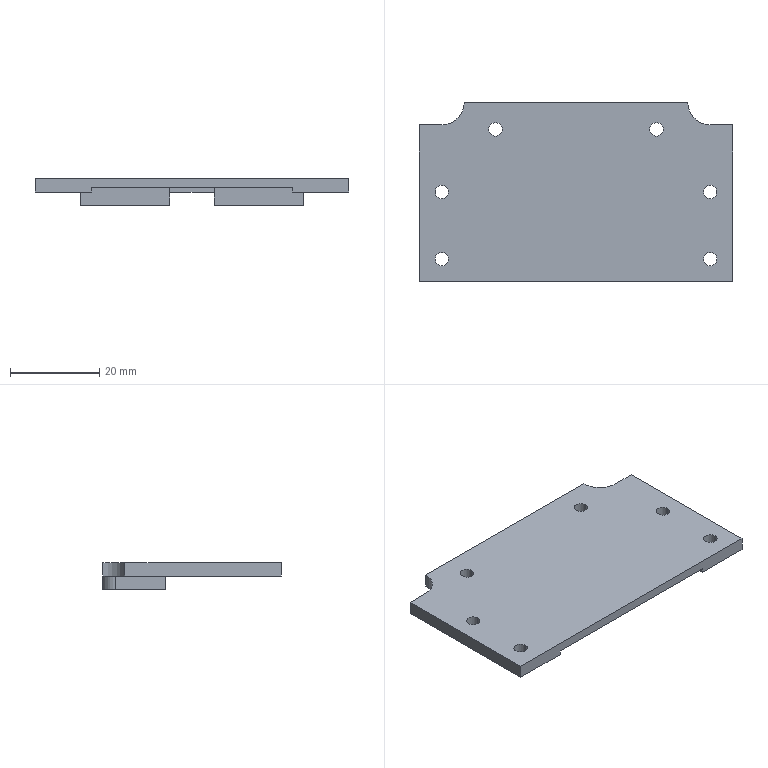Part | SolidWorks | features ICE 2, MBimport 1 | 1 solid | 48 faces | box 70 x 40 x 6 mm | volume 8316 mm3 | plane 28 | cylinder 20 | commonest cylinder face diameters 3 x16 6 x2 10 x2
STEP:
#1=CARTESIAN_POINT('',(-8.5,14.,1.));
#2=VERTEX_POINT('',#1);
#3=CARTESIAN_POINT('',(-11.5,14.,1.));
#4=VERTEX_POINT('',#3);
#5=CARTESIAN_POINT('',(-10.,14.,1.));
#6=DIRECTION('',(0.,0.,-1.));
#7=DIRECTION('',(-1.,0.,0.));
#8=AXIS2_PLACEMENT_3D('',#5,#6,#7);
#9=CIRCLE('',#8,1.5);
#10=EDGE_CURVE('',#2,#4,#9,.T.);
#11=ORIENTED_EDGE('',*,*,#10,.F.);
#12=CARTESIAN_POINT('',(-8.5,14.,-3.));
#13=VERTEX_POINT('',#12);
#14=CARTESIAN_POINT('',(-8.5,14.,3.002));
#15=DIRECTION('',(0.,0.,-1.));
#16=VECTOR('',#15,1000.);
#17=LINE('',#14,#16);
#18=EDGE_CURVE('',#2,#13,#17,.T.);
#19=ORIENTED_EDGE('',*,*,#18,.T.);
#20=CARTESIAN_POINT('',(-11.5,14.,-3.));
#21=VERTEX_POINT('',#20);
#22=CARTESIAN_POINT('',(-10.,14.,-3.));
#23=DIRECTION('',(0.,0.,1.));
#24=DIRECTION('',(-1.,0.,0.));
#25=AXIS2_PLACEMENT_3D('',#22,#23,#24);
#26=CIRCLE('',#25,1.5);
#27=EDGE_CURVE('',#21,#13,#26,.T.);
#28=ORIENTED_EDGE('',*,*,#27,.F.);
#29=CARTESIAN_POINT('',(-11.5,14.,3.002));
#30=DIRECTION('',(0.,0.,-1.));
#31=VECTOR('',#30,1000.);
#32=LINE('',#29,#31);
#33=EDGE_CURVE('',#4,#21,#32,.T.);
#34=ORIENTED_EDGE('',*,*,#33,.F.);
#35=EDGE_LOOP('',(#11,#19,#28,#34));
#36=FACE_OUTER_BOUND('',#35,.T.);
#37=CARTESIAN_POINT('',(-10.,14.,3.002));
#38=DIRECTION('',(0.,0.,-1.));
#39=DIRECTION('',(-1.,0.,0.));
#40=AXIS2_PLACEMENT_3D('',#37,#38,#39);
#41=CYLINDRICAL_SURFACE('',#40,1.5);
#42=ADVANCED_FACE('',(#36),#41,.F.);
#43=CARTESIAN_POINT('',(8.5,14.,1.));
#44=VERTEX_POINT('',#43);
#45=CARTESIAN_POINT('',(11.5,14.,1.));
#46=VERTEX_POINT('',#45);
#47=CARTESIAN_POINT('',(10.,14.,1.));
#48=DIRECTION('',(0.,0.,1.));
#49=DIRECTION('',(-1.,0.,0.));
#50=AXIS2_PLACEMENT_3D('',#47,#48,#49);
#51=CIRCLE('',#50,1.5);
#52=EDGE_CURVE('',#44,#46,#51,.T.);
#53=ORIENTED_EDGE('',*,*,#52,.T.);
#54=CARTESIAN_POINT('',(11.5,14.,-3.));
#55=VERTEX_POINT('',#54);
#56=CARTESIAN_POINT('',(11.5,14.,3.002));
#57=DIRECTION('',(0.,0.,-1.));
#58=VECTOR('',#57,1000.);
#59=LINE('',#56,#58);
#60=EDGE_CURVE('',#46,#55,#59,.T.);
#61=ORIENTED_EDGE('',*,*,#60,.T.);
#62=CARTESIAN_POINT('',(8.5,14.,-3.));
#63=VERTEX_POINT('',#62);
#64=CARTESIAN_POINT('',(10.,14.,-3.));
#65=DIRECTION('',(0.,0.,-1.));
#66=DIRECTION('',(-1.,0.,0.));
#67=AXIS2_PLACEMENT_3D('',#64,#65,#66);
#68=CIRCLE('',#67,1.5);
#69=EDGE_CURVE('',#55,#63,#68,.T.);
#70=ORIENTED_EDGE('',*,*,#69,.T.);
#71=CARTESIAN_POINT('',(8.5,14.,3.002));
#72=DIRECTION('',(0.,0.,-1.));
#73=VECTOR('',#72,1000.);
#74=LINE('',#71,#73);
#75=EDGE_CURVE('',#44,#63,#74,.T.);
#76=ORIENTED_EDGE('',*,*,#75,.F.);
#77=EDGE_LOOP('',(#53,#61,#70,#76));
#78=FACE_OUTER_BOUND('',#77,.T.);
#79=CARTESIAN_POINT('',(10.,14.,3.002));
#80=DIRECTION('',(0.,0.,-1.));
#81=DIRECTION('',(-1.,0.,0.));
#82=AXIS2_PLACEMENT_3D('',#79,#80,#81);
#83=CYLINDRICAL_SURFACE('',#82,1.5);
#84=ADVANCED_FACE('',(#78),#83,.F.);
#85=CARTESIAN_POINT('',(-22.5,6.,1.));
#86=VERTEX_POINT('',#85);
#87=CARTESIAN_POINT('',(-5.,6.,1.));
#88=VERTEX_POINT('',#87);
#89=CARTESIAN_POINT('',(-22.5,6.,1.));
#90=DIRECTION('',(1.,0.,0.));
#91=VECTOR('',#90,1000.);
#92=LINE('',#89,#91);
#93=EDGE_CURVE('',#86,#88,#92,.T.);
#94=ORIENTED_EDGE('',*,*,#93,.T.);
#95=CARTESIAN_POINT('',(-5.,15.,1.));
#96=VERTEX_POINT('',#95);
#97=CARTESIAN_POINT('',(-5.,0.,1.));
#98=DIRECTION('',(0.,-1.,0.));
#99=VECTOR('',#98,1000.);
#100=LINE('',#97,#99);
#101=EDGE_CURVE('',#96,#88,#100,.T.);
#102=ORIENTED_EDGE('',*,*,#101,.F.);
#103=CARTESIAN_POINT('',(5.,15.,1.));
#104=VERTEX_POINT('',#103);
#105=CARTESIAN_POINT('',(-15.,15.,1.));
#106=DIRECTION('',(1.,0.,0.));
#107=VECTOR('',#106,1000.);
#108=LINE('',#105,#107);
#109=EDGE_CURVE('',#96,#104,#108,.T.);
#110=ORIENTED_EDGE('',*,*,#109,.T.);
#111=CARTESIAN_POINT('',(5.,6.,1.));
#112=VERTEX_POINT('',#111);
#113=CARTESIAN_POINT('',(5.,0.,1.));
#114=DIRECTION('',(0.,-1.,0.));
#115=VECTOR('',#114,1000.);
#116=LINE('',#113,#115);
#117=EDGE_CURVE('',#104,#112,#116,.T.);
#118=ORIENTED_EDGE('',*,*,#117,.T.);
#119=CARTESIAN_POINT('',(22.5,6.,1.));
#120=VERTEX_POINT('',#119);
#121=CARTESIAN_POINT('',(22.5,6.,1.));
#122=DIRECTION('',(-1.,0.,0.));
#123=VECTOR('',#122,1000.);
#124=LINE('',#121,#123);
#125=EDGE_CURVE('',#120,#112,#124,.T.);
#126=ORIENTED_EDGE('',*,*,#125,.F.);
#127=CARTESIAN_POINT('',(22.5,-20.,1.));
#128=VERTEX_POINT('',#127);
#129=CARTESIAN_POINT('',(22.5,6.,1.));
#130=DIRECTION('',(0.,-1.,0.));
#131=VECTOR('',#130,1000.);
#132=LINE('',#129,#131);
#133=EDGE_CURVE('',#120,#128,#132,.T.);
#134=ORIENTED_EDGE('',*,*,#133,.T.);
#135=CARTESIAN_POINT('',(-22.5,-20.,1.));
#136=VERTEX_POINT('',#135);
#137=CARTESIAN_POINT('',(22.5,-20.,1.));
#138=DIRECTION('',(-1.,0.,0.));
#139=VECTOR('',#138,1000.);
#140=LINE('',#137,#139);
#141=EDGE_CURVE('',#128,#136,#140,.T.);
#142=ORIENTED_EDGE('',*,*,#141,.T.);
#143=CARTESIAN_POINT('',(-22.5,-20.,1.));
#144=DIRECTION('',(0.,1.,0.));
#145=VECTOR('',#144,1000.);
#146=LINE('',#143,#145);
#147=EDGE_CURVE('',#136,#86,#146,.T.);
#148=ORIENTED_EDGE('',*,*,#147,.T.);
#149=EDGE_LOOP('',(#94,#102,#110,#118,#126,#134,#142,#148));
#150=FACE_OUTER_BOUND('',#149,.T.);
#151=CARTESIAN_POINT('',(0.,0.,1.));
#152=DIRECTION('',(0.,0.,-1.));
#153=DIRECTION('',(-1.,0.,0.));
#154=AXIS2_PLACEMENT_3D('',#151,#152,#153);
#155=PLANE('',#154);
#156=ADVANCED_FACE('',(#150),#155,.T.);
#157=CARTESIAN_POINT('',(-5.,15.,0.));
#158=VERTEX_POINT('',#157);
#159=CARTESIAN_POINT('',(-5.,20.,0.));
#160=VERTEX_POINT('',#159);
#161=CARTESIAN_POINT('',(-5.,0.,0.));
#162=DIRECTION('',(0.,1.,0.));
#163=VECTOR('',#162,1000.);
#164=LINE('',#161,#163);
#165=EDGE_CURVE('',#158,#160,#164,.T.);
#166=ORIENTED_EDGE('',*,*,#165,.T.);
#167=CARTESIAN_POINT('',(5.,20.,0.));
#168=VERTEX_POINT('',#167);
#169=CARTESIAN_POINT('',(15.,20.,0.));
#170=DIRECTION('',(-1.,0.,0.));
#171=VECTOR('',#170,1000.);
#172=LINE('',#169,#171);
#173=EDGE_CURVE('',#168,#160,#172,.T.);
#174=ORIENTED_EDGE('',*,*,#173,.F.);
#175=CARTESIAN_POINT('',(5.,15.,0.));
#176=VERTEX_POINT('',#175);
#177=CARTESIAN_POINT('',(5.,0.,0.));
#178=DIRECTION('',(0.,1.,0.));
#179=VECTOR('',#178,1000.);
#180=LINE('',#177,#179);
#181=EDGE_CURVE('',#176,#168,#180,.T.);
#182=ORIENTED_EDGE('',*,*,#181,.F.);
#183=CARTESIAN_POINT('',(-15.,15.,0.));
#184=DIRECTION('',(1.,0.,0.));
#185=VECTOR('',#184,1000.);
#186=LINE('',#183,#185);
#187=EDGE_CURVE('',#158,#176,#186,.T.);
#188=ORIENTED_EDGE('',*,*,#187,.F.);
#189=EDGE_LOOP('',(#166,#174,#182,#188));
#190=FACE_OUTER_BOUND('',#189,.T.);
#191=CARTESIAN_POINT('',(0.,0.,0.));
#192=DIRECTION('',(0.,0.,1.));
#193=DIRECTION('',(0.,-1.,0.));
#194=AXIS2_PLACEMENT_3D('',#191,#192,#193);
#195=PLANE('',#194);
#196=ADVANCED_FACE('',(#190),#195,.F.);
#197=CARTESIAN_POINT('',(-5.,15.,3.002));
#198=DIRECTION('',(0.,0.,-1.));
#199=VECTOR('',#198,1000.);
#200=LINE('',#197,#199);
#201=EDGE_CURVE('',#96,#158,#200,.T.);
#202=ORIENTED_EDGE('',*,*,#201,.T.);
#203=ORIENTED_EDGE('',*,*,#187,.T.);
#204=CARTESIAN_POINT('',(5.,15.,3.002));
#205=DIRECTION('',(0.,0.,-1.));
#206=VECTOR('',#205,1000.);
#207=LINE('',#204,#206);
#208=EDGE_CURVE('',#104,#176,#207,.T.);
#209=ORIENTED_EDGE('',*,*,#208,.F.);
#210=ORIENTED_EDGE('',*,*,#109,.F.);
#211=EDGE_LOOP('',(#202,#203,#209,#210));
#212=FACE_OUTER_BOUND('',#211,.T.);
#213=CARTESIAN_POINT('',(-22.5,15.,0.));
#214=DIRECTION('',(0.,1.,0.));
#215=DIRECTION('',(1.,0.,0.));
#216=AXIS2_PLACEMENT_3D('',#213,#214,#215);
#217=PLANE('',#216);
#218=ADVANCED_FACE('',(#212),#217,.F.);
#219=CARTESIAN_POINT('',(-31.5,0.,0.));
#220=VERTEX_POINT('',#219);
#221=CARTESIAN_POINT('',(-28.5,0.,0.));
#222=VERTEX_POINT('',#221);
#223=CARTESIAN_POINT('',(-30.,0.,0.));
#224=DIRECTION('',(0.,0.,1.));
#225=DIRECTION('',(-1.,0.,0.));
#226=AXIS2_PLACEMENT_3D('',#223,#224,#225);
#227=CIRCLE('',#226,1.5);
#228=EDGE_CURVE('',#220,#222,#227,.T.);
#229=ORIENTED_EDGE('',*,*,#228,.T.);
#230=CARTESIAN_POINT('',(-30.,0.,0.));
#231=DIRECTION('',(0.,0.,1.));
#232=DIRECTION('',(1.,0.,0.));
#233=AXIS2_PLACEMENT_3D('',#230,#231,#232);
#234=CIRCLE('',#233,1.5);
#235=EDGE_CURVE('',#222,#220,#234,.T.);
#236=ORIENTED_EDGE('',*,*,#235,.T.);
#237=EDGE_LOOP('',(#229,#236));
#238=FACE_BOUND('',#237,.T.);
#239=CARTESIAN_POINT('',(-25.,6.,0.));
#240=VERTEX_POINT('',#239);
#241=CARTESIAN_POINT('',(-22.5,6.,0.));
#242=VERTEX_POINT('',#241);
#243=CARTESIAN_POINT('',(-25.,6.,0.));
#244=DIRECTION('',(1.,0.,0.));
#245=VECTOR('',#244,1000.);
#246=LINE('',#243,#245);
#247=EDGE_CURVE('',#240,#242,#246,.T.);
#248=ORIENTED_EDGE('',*,*,#247,.T.);
#249=CARTESIAN_POINT('',(-22.5,-20.,0.));
#250=VERTEX_POINT('',#249);
#251=CARTESIAN_POINT('',(-22.5,-17.,0.));
#252=DIRECTION('',(0.,1.,0.));
#253=VECTOR('',#252,1000.);
#254=LINE('',#251,#253);
#255=EDGE_CURVE('',#250,#242,#254,.T.);
#256=ORIENTED_EDGE('',*,*,#255,.F.);
#257=CARTESIAN_POINT('',(-35.,-20.,0.));
#258=VERTEX_POINT('',#257);
#259=CARTESIAN_POINT('',(-35.,-20.,0.));
#260=DIRECTION('',(-1.,0.,0.));
#261=VECTOR('',#260,1000.);
#262=LINE('',#259,#261);
#263=EDGE_CURVE('',#250,#258,#262,.T.);
#264=ORIENTED_EDGE('',*,*,#263,.T.);
#265=CARTESIAN_POINT('',(-35.,15.,0.));
#266=VERTEX_POINT('',#265);
#267=CARTESIAN_POINT('',(-35.,15.,0.));
#268=DIRECTION('',(0.,-1.,0.));
#269=VECTOR('',#268,1000.);
#270=LINE('',#267,#269);
#271=EDGE_CURVE('',#266,#258,#270,.T.);
#272=ORIENTED_EDGE('',*,*,#271,.F.);
#273=CARTESIAN_POINT('',(-30.,15.,0.));
#274=VERTEX_POINT('',#273);
#275=CARTESIAN_POINT('',(-35.,15.,0.));
#276=DIRECTION('',(1.,0.,0.));
#277=VECTOR('',#276,1000.);
#278=LINE('',#275,#277);
#279=EDGE_CURVE('',#266,#274,#278,.T.);
#280=ORIENTED_EDGE('',*,*,#279,.T.);
#281=CARTESIAN_POINT('',(-25.,20.,0.));
#282=VERTEX_POINT('',#281);
#283=CARTESIAN_POINT('',(-30.,20.,0.));
#284=DIRECTION('',(0.,0.,1.));
#285=DIRECTION('',(0.,-1.,0.));
#286=AXIS2_PLACEMENT_3D('',#283,#284,#285);
#287=CIRCLE('',#286,5.);
#288=EDGE_CURVE('',#274,#282,#287,.T.);
#289=ORIENTED_EDGE('',*,*,#288,.T.);
#290=CARTESIAN_POINT('',(-22.,20.,0.));
#291=VERTEX_POINT('',#290);
#292=CARTESIAN_POINT('',(-22.,20.,0.));
#293=DIRECTION('',(-1.,0.,0.));
#294=VECTOR('',#293,1000.);
#295=LINE('',#292,#294);
#296=EDGE_CURVE('',#291,#282,#295,.T.);
#297=ORIENTED_EDGE('',*,*,#296,.F.);
#298=CARTESIAN_POINT('',(-25.,17.,0.));
#299=VERTEX_POINT('',#298);
#300=CARTESIAN_POINT('',(-22.,17.,0.));
#301=DIRECTION('',(0.,0.,1.));
#302=DIRECTION('',(0.,1.,0.));
#303=AXIS2_PLACEMENT_3D('',#300,#301,#302);
#304=CIRCLE('',#303,3.);
#305=EDGE_CURVE('',#291,#299,#304,.T.);
#306=ORIENTED_EDGE('',*,*,#305,.T.);
#307=CARTESIAN_POINT('',(-25.,17.,0.));
#308=DIRECTION('',(0.,-1.,0.));
#309=VECTOR('',#308,1000.);
#310=LINE('',#307,#309);
#311=EDGE_CURVE('',#299,#240,#310,.T.);
#312=ORIENTED_EDGE('',*,*,#311,.T.);
#313=EDGE_LOOP('',(#248,#256,#264,#272,#280,#289,#297,#306,#312));
#314=FACE_OUTER_BOUND('',#313,.T.);
#315=CARTESIAN_POINT('',(-31.5,-15.,0.));
#316=VERTEX_POINT('',#315);
#317=CARTESIAN_POINT('',(-28.5,-15.,0.));
#318=VERTEX_POINT('',#317);
#319=CARTESIAN_POINT('',(-30.,-15.,0.));
#320=DIRECTION('',(0.,0.,-1.));
#321=DIRECTION('',(1.,0.,0.));
#322=AXIS2_PLACEMENT_3D('',#319,#320,#321);
#323=CIRCLE('',#322,1.5);
#324=EDGE_CURVE('',#316,#318,#323,.T.);
#325=ORIENTED_EDGE('',*,*,#324,.F.);
#326=CARTESIAN_POINT('',(-30.,-15.,0.));
#327=DIRECTION('',(0.,0.,-1.));
#328=DIRECTION('',(1.,0.,0.));
#329=AXIS2_PLACEMENT_3D('',#326,#327,#328);
#330=CIRCLE('',#329,1.5);
#331=EDGE_CURVE('',#318,#316,#330,.T.);
#332=ORIENTED_EDGE('',*,*,#331,.F.);
#333=EDGE_LOOP('',(#325,#332));
#334=FACE_BOUND('',#333,.T.);
#335=CARTESIAN_POINT('',(0.,0.,0.));
#336=DIRECTION('',(0.,0.,1.));
#337=DIRECTION('',(0.,-1.,0.));
#338=AXIS2_PLACEMENT_3D('',#335,#336,#337);
#339=PLANE('',#338);
#340=ADVANCED_FACE('',(#238,#314,#334),#339,.F.);
#341=ORIENTED_EDGE('',*,*,#228,.F.);
#342=CARTESIAN_POINT('',(-31.5,0.,3.));
#343=VERTEX_POINT('',#342);
#344=CARTESIAN_POINT('',(-31.5,0.,0.));
#345=DIRECTION('',(0.,0.,1.));
#346=VECTOR('',#345,1000.);
#347=LINE('',#344,#346);
#348=EDGE_CURVE('',#220,#343,#347,.T.);
#349=ORIENTED_EDGE('',*,*,#348,.T.);
#350=CARTESIAN_POINT('',(-28.5,0.,3.));
#351=VERTEX_POINT('',#350);
#352=CARTESIAN_POINT('',(-30.,0.,3.));
#353=DIRECTION('',(0.,0.,1.));
#354=DIRECTION('',(-1.,0.,0.));
#355=AXIS2_PLACEMENT_3D('',#352,#353,#354);
#356=CIRCLE('',#355,1.5);
#357=EDGE_CURVE('',#343,#351,#356,.T.);
#358=ORIENTED_EDGE('',*,*,#357,.T.);
#359=CARTESIAN_POINT('',(-28.5,0.,0.));
#360=DIRECTION('',(0.,0.,1.));
#361=VECTOR('',#360,1000.);
#362=LINE('',#359,#361);
#363=EDGE_CURVE('',#222,#351,#362,.T.);
#364=ORIENTED_EDGE('',*,*,#363,.F.);
#365=EDGE_LOOP('',(#341,#349,#358,#364));
#366=FACE_OUTER_BOUND('',#365,.T.);
#367=CARTESIAN_POINT('',(-30.,0.,0.));
#368=DIRECTION('',(0.,0.,-1.));
#369=DIRECTION('',(1.,0.,0.));
#370=AXIS2_PLACEMENT_3D('',#367,#368,#369);
#371=CYLINDRICAL_SURFACE('',#370,1.5);
#372=ADVANCED_FACE('',(#366),#371,.F.);
#373=CARTESIAN_POINT('',(-30.,0.,3.));
#374=DIRECTION('',(0.,0.,1.));
#375=DIRECTION('',(1.,0.,0.));
#376=AXIS2_PLACEMENT_3D('',#373,#374,#375);
#377=CIRCLE('',#376,1.5);
#378=EDGE_CURVE('',#351,#343,#377,.T.);
#379=ORIENTED_EDGE('',*,*,#378,.T.);
#380=ORIENTED_EDGE('',*,*,#348,.F.);
#381=ORIENTED_EDGE('',*,*,#235,.F.);
#382=ORIENTED_EDGE('',*,*,#363,.T.);
#383=EDGE_LOOP('',(#379,#380,#381,#382));
#384=FACE_OUTER_BOUND('',#383,.T.);
#385=CARTESIAN_POINT('',(-30.,0.,0.));
#386=DIRECTION('',(0.,0.,-1.));
#387=DIRECTION('',(1.,0.,0.));
#388=AXIS2_PLACEMENT_3D('',#385,#386,#387);
#389=CYLINDRICAL_SURFACE('',#388,1.5);
#390=ADVANCED_FACE('',(#384),#389,.F.);
#391=CARTESIAN_POINT('',(-25.,6.,-3.));
#392=VERTEX_POINT('',#391);
#393=CARTESIAN_POINT('',(-5.,6.,-3.));
#394=VERTEX_POINT('',#393);
#395=CARTESIAN_POINT('',(-25.,6.,-3.));
#396=DIRECTION('',(1.,0.,0.));
#397=VECTOR('',#396,1000.);
#398=LINE('',#395,#397);
#399=EDGE_CURVE('',#392,#394,#398,.T.);
#400=ORIENTED_EDGE('',*,*,#399,.T.);
#401=CARTESIAN_POINT('',(-5.,6.,3.002));
#402=DIRECTION('',(0.,0.,-1.));
#403=VECTOR('',#402,1000.);
#404=LINE('',#401,#403);
#405=EDGE_CURVE('',#88,#394,#404,.T.);
#406=ORIENTED_EDGE('',*,*,#405,.F.);
#407=ORIENTED_EDGE('',*,*,#93,.F.);
#408=CARTESIAN_POINT('',(-22.5,6.,1.));
#409=DIRECTION('',(0.,0.,-1.));
#410=VECTOR('',#409,1000.);
#411=LINE('',#408,#410);
#412=EDGE_CURVE('',#86,#242,#411,.T.);
#413=ORIENTED_EDGE('',*,*,#412,.T.);
#414=ORIENTED_EDGE('',*,*,#247,.F.);
#415=CARTESIAN_POINT('',(-25.,6.,0.));
#416=DIRECTION('',(0.,0.,-1.));
#417=VECTOR('',#416,1000.);
#418=LINE('',#415,#417);
#419=EDGE_CURVE('',#240,#392,#418,.T.);
#420=ORIENTED_EDGE('',*,*,#419,.T.);
#421=EDGE_LOOP('',(#400,#406,#407,#413,#414,#420));
#422=FACE_OUTER_BOUND('',#421,.T.);
#423=CARTESIAN_POINT('',(-25.,6.,1.));
#424=DIRECTION('',(0.,1.,0.));
#425=DIRECTION('',(1.,0.,0.));
#426=AXIS2_PLACEMENT_3D('',#423,#424,#425);
#427=PLANE('',#426);
#428=ADVANCED_FACE('',(#422),#427,.F.);
#429=CARTESIAN_POINT('',(-22.5,-20.,-6.));
#430=DIRECTION('',(0.,0.,1.));
#431=VECTOR('',#430,1000.);
#432=LINE('',#429,#431);
#433=EDGE_CURVE('',#250,#136,#432,.T.);
#434=ORIENTED_EDGE('',*,*,#433,.F.);
#435=ORIENTED_EDGE('',*,*,#255,.T.);
#436=ORIENTED_EDGE('',*,*,#412,.F.);
#437=ORIENTED_EDGE('',*,*,#147,.F.);
#438=EDGE_LOOP('',(#434,#435,#436,#437));
#439=FACE_OUTER_BOUND('',#438,.T.);
#440=CARTESIAN_POINT('',(-22.5,-20.,0.));
#441=DIRECTION('',(-1.,0.,0.));
#442=DIRECTION('',(0.,1.,0.));
#443=AXIS2_PLACEMENT_3D('',#440,#441,#442);
#444=PLANE('',#443);
#445=ADVANCED_FACE('',(#439),#444,.F.);
#446=ORIENTED_EDGE('',*,*,#271,.T.);
#447=CARTESIAN_POINT('',(-35.,-20.,3.));
#448=VERTEX_POINT('',#447);
#449=CARTESIAN_POINT('',(-35.,-20.,3.));
#450=DIRECTION('',(0.,0.,-1.));
#451=VECTOR('',#450,1000.);
#452=LINE('',#449,#451);
#453=EDGE_CURVE('',#448,#258,#452,.T.);
#454=ORIENTED_EDGE('',*,*,#453,.F.);
#455=CARTESIAN_POINT('',(-35.,15.,3.));
#456=VERTEX_POINT('',#455);
#457=CARTESIAN_POINT('',(-35.,15.,3.));
#458=DIRECTION('',(0.,-1.,0.));
#459=VECTOR('',#458,1000.);
#460=LINE('',#457,#459);
#461=EDGE_CURVE('',#456,#448,#460,.T.);
#462=ORIENTED_EDGE('',*,*,#461,.F.);
#463=CARTESIAN_POINT('',(-35.,15.,3.));
#464=DIRECTION('',(0.,0.,-1.));
#465=VECTOR('',#464,1000.);
#466=LINE('',#463,#465);
#467=EDGE_CURVE('',#456,#266,#466,.T.);
#468=ORIENTED_EDGE('',*,*,#467,.T.);
#469=EDGE_LOOP('',(#446,#454,#462,#468));
#470=FACE_OUTER_BOUND('',#469,.T.);
#471=CARTESIAN_POINT('',(-35.,20.,0.));
#472=DIRECTION('',(-1.,0.,0.));
#473=DIRECTION('',(0.,-1.,0.));
#474=AXIS2_PLACEMENT_3D('',#471,#472,#473);
#475=PLANE('',#474);
#476=ADVANCED_FACE('',(#470),#475,.T.);
#477=ORIENTED_EDGE('',*,*,#279,.F.);
#478=ORIENTED_EDGE('',*,*,#467,.F.);
#479=CARTESIAN_POINT('',(-30.,15.,3.));
#480=VERTEX_POINT('',#479);
#481=CARTESIAN_POINT('',(-35.,15.,3.));
#482=DIRECTION('',(1.,0.,0.));
#483=VECTOR('',#482,1000.);
#484=LINE('',#481,#483);
#485=EDGE_CURVE('',#456,#480,#484,.T.);
#486=ORIENTED_EDGE('',*,*,#485,.T.);
#487=CARTESIAN_POINT('',(-30.,15.,3.));
#488=DIRECTION('',(0.,0.,-1.));
#489=VECTOR('',#488,1000.);
#490=LINE('',#487,#489);
#491=EDGE_CURVE('',#480,#274,#490,.T.);
#492=ORIENTED_EDGE('',*,*,#491,.T.);
#493=EDGE_LOOP('',(#477,#478,#486,#492));
#494=FACE_OUTER_BOUND('',#493,.T.);
#495=CARTESIAN_POINT('',(-35.,15.,0.));
#496=DIRECTION('',(0.,1.,0.));
#497=DIRECTION('',(1.,0.,0.));
#498=AXIS2_PLACEMENT_3D('',#495,#496,#497);
#499=PLANE('',#498);
#500=ADVANCED_FACE('',(#494),#499,.T.);
#501=ORIENTED_EDGE('',*,*,#491,.F.);
#502=CARTESIAN_POINT('',(-25.,20.,3.));
#503=VERTEX_POINT('',#502);
#504=CARTESIAN_POINT('',(-30.,20.,3.));
#505=DIRECTION('',(0.,0.,-1.));
#506=DIRECTION('',(1.,0.,0.));
#507=AXIS2_PLACEMENT_3D('',#504,#505,#506);
#508=CIRCLE('',#507,5.);
#509=EDGE_CURVE('',#503,#480,#508,.T.);
#510=ORIENTED_EDGE('',*,*,#509,.F.);
#511=CARTESIAN_POINT('',(-25.,20.,3.));
#512=DIRECTION('',(0.,0.,-1.));
#513=VECTOR('',#512,1000.);
#514=LINE('',#511,#513);
#515=EDGE_CURVE('',#503,#282,#514,.T.);
#516=ORIENTED_EDGE('',*,*,#515,.T.);
#517=ORIENTED_EDGE('',*,*,#288,.F.);
#518=EDGE_LOOP('',(#501,#510,#516,#517));
#519=FACE_OUTER_BOUND('',#518,.T.);
#520=CARTESIAN_POINT('',(-30.,20.,14.732));
#521=DIRECTION('',(0.,0.,1.));
#522=DIRECTION('',(1.,0.,0.));
#523=AXIS2_PLACEMENT_3D('',#520,#521,#522);
#524=CYLINDRICAL_SURFACE('',#523,5.);
#525=ADVANCED_FACE('',(#519),#524,.F.);
#526=CARTESIAN_POINT('',(-5.,20.,-3.));
#527=VERTEX_POINT('',#526);
#528=CARTESIAN_POINT('',(-5.,20.,3.002));
#529=DIRECTION('',(0.,0.,-1.));
#530=VECTOR('',#529,1000.);
#531=LINE('',#528,#530);
#532=EDGE_CURVE('',#160,#527,#531,.T.);
#533=ORIENTED_EDGE('',*,*,#532,.T.);
#534=CARTESIAN_POINT('',(-22.,20.,-3.));
#535=VERTEX_POINT('',#534);
#536=CARTESIAN_POINT('',(-15.,20.,-3.));
#537=DIRECTION('',(-1.,0.,0.));
#538=VECTOR('',#537,1000.);
#539=LINE('',#536,#538);
#540=EDGE_CURVE('',#527,#535,#539,.T.);
#541=ORIENTED_EDGE('',*,*,#540,.T.);
#542=CARTESIAN_POINT('',(-22.,20.,0.));
#543=DIRECTION('',(0.,0.,-1.));
#544=VECTOR('',#543,1000.);
#545=LINE('',#542,#544);
#546=EDGE_CURVE('',#291,#535,#545,.T.);
#547=ORIENTED_EDGE('',*,*,#546,.F.);
#548=ORIENTED_EDGE('',*,*,#296,.T.);
#549=ORIENTED_EDGE('',*,*,#515,.F.);
#550=CARTESIAN_POINT('',(25.,20.,3.));
#551=VERTEX_POINT('',#550);
#552=CARTESIAN_POINT('',(25.,20.,3.));
#553=DIRECTION('',(-1.,0.,0.));
#554=VECTOR('',#553,1000.);
#555=LINE('',#552,#554);
#556=EDGE_CURVE('',#551,#503,#555,.T.);
#557=ORIENTED_EDGE('',*,*,#556,.F.);
#558=CARTESIAN_POINT('',(25.,20.,0.));
#559=VERTEX_POINT('',#558);
#560=CARTESIAN_POINT('',(25.,20.,0.));
#561=DIRECTION('',(0.,0.,1.));
#562=VECTOR('',#561,1000.);
#563=LINE('',#560,#562);
#564=EDGE_CURVE('',#559,#551,#563,.T.);
#565=ORIENTED_EDGE('',*,*,#564,.F.);
#566=CARTESIAN_POINT('',(22.,20.,0.));
#567=VERTEX_POINT('',#566);
#568=CARTESIAN_POINT('',(22.,20.,0.));
#569=DIRECTION('',(1.,0.,0.));
#570=VECTOR('',#569,1000.);
#571=LINE('',#568,#570);
#572=EDGE_CURVE('',#567,#559,#571,.T.);
#573=ORIENTED_EDGE('',*,*,#572,.F.);
#574=CARTESIAN_POINT('',(22.,20.,-3.));
#575=VERTEX_POINT('',#574);
#576=CARTESIAN_POINT('',(22.,20.,-3.));
#577=DIRECTION('',(0.,0.,1.));
#578=VECTOR('',#577,1000.);
#579=LINE('',#576,#578);
#580=EDGE_CURVE('',#575,#567,#579,.T.);
#581=ORIENTED_EDGE('',*,*,#580,.F.);
#582=CARTESIAN_POINT('',(5.,20.,-3.));
#583=VERTEX_POINT('',#582);
#584=CARTESIAN_POINT('',(15.,20.,-3.));
#585=DIRECTION('',(1.,0.,0.));
#586=VECTOR('',#585,1000.);
#587=LINE('',#584,#586);
#588=EDGE_CURVE('',#583,#575,#587,.T.);
#589=ORIENTED_EDGE('',*,*,#588,.F.);
#590=CARTESIAN_POINT('',(5.,20.,3.002));
#591=DIRECTION('',(0.,0.,-1.));
#592=VECTOR('',#591,1000.);
#593=LINE('',#590,#592);
#594=EDGE_CURVE('',#168,#583,#593,.T.);
#595=ORIENTED_EDGE('',*,*,#594,.F.);
#596=ORIENTED_EDGE('',*,*,#173,.T.);
#597=EDGE_LOOP('',(#533,#541,#547,#548,#549,#557,#565,#573,#581,#589,#595,#596));
#598=FACE_OUTER_BOUND('',#597,.T.);
#599=CARTESIAN_POINT('',(35.,20.,0.));
#600=DIRECTION('',(0.,1.,0.));
#601=DIRECTION('',(-1.,0.,0.));
#602=AXIS2_PLACEMENT_3D('',#599,#600,#601);
#603=PLANE('',#602);
#604=ADVANCED_FACE('',(#598),#603,.T.);
#605=CARTESIAN_POINT('',(-25.,17.,-3.));
#606=VERTEX_POINT('',#605);
#607=CARTESIAN_POINT('',(-25.,17.,0.));
#608=DIRECTION('',(0.,0.,-1.));
#609=VECTOR('',#608,1000.);
#610=LINE('',#607,#609);
#611=EDGE_CURVE('',#299,#606,#610,.T.);
#612=ORIENTED_EDGE('',*,*,#611,.F.);
#613=ORIENTED_EDGE('',*,*,#305,.F.);
#614=ORIENTED_EDGE('',*,*,#546,.T.);
#615=CARTESIAN_POINT('',(-22.,17.,-3.));
#616=DIRECTION('',(0.,0.,-1.));
#617=DIRECTION('',(-1.,0.,0.));
#618=AXIS2_PLACEMENT_3D('',#615,#616,#617);
#619=CIRCLE('',#618,3.);
#620=EDGE_CURVE('',#606,#535,#619,.T.);
#621=ORIENTED_EDGE('',*,*,#620,.F.);
#622=EDGE_LOOP('',(#612,#613,#614,#621));
#623=FACE_OUTER_BOUND('',#622,.T.);
#624=CARTESIAN_POINT('',(-22.,17.,14.732));
#625=DIRECTION('',(0.,0.,1.));
#626=DIRECTION('',(-1.,0.,0.));
#627=AXIS2_PLACEMENT_3D('',#624,#625,#626);
#628=CYLINDRICAL_SURFACE('',#627,3.);
#629=ADVANCED_FACE('',(#623),#628,.T.);
#630=ORIENTED_EDGE('',*,*,#419,.F.);
#631=ORIENTED_EDGE('',*,*,#311,.F.);
#632=ORIENTED_EDGE('',*,*,#611,.T.);
#633=CARTESIAN_POINT('',(-25.,17.,-3.));
#634=DIRECTION('',(0.,-1.,0.));
#635=VECTOR('',#634,1000.);
#636=LINE('',#633,#635);
#637=EDGE_CURVE('',#606,#392,#636,.T.);
#638=ORIENTED_EDGE('',*,*,#637,.T.);
#639=EDGE_LOOP('',(#630,#631,#632,#638));
#640=FACE_OUTER_BOUND('',#639,.T.);
#641=CARTESIAN_POINT('',(-25.,20.,1.));
#642=DIRECTION('',(1.,0.,0.));
#643=DIRECTION('',(0.,-1.,0.));
#644=AXIS2_PLACEMENT_3D('',#641,#642,#643);
#645=PLANE('',#644);
#646=ADVANCED_FACE('',(#640),#645,.F.);
#647=CARTESIAN_POINT('',(-19.5,14.,3.));
#648=VERTEX_POINT('',#647);
#649=CARTESIAN_POINT('',(-16.5,14.,3.));
#650=VERTEX_POINT('',#649);
#651=CARTESIAN_POINT('',(-18.,14.,3.));
#652=DIRECTION('',(0.,0.,1.));
#653=DIRECTION('',(-1.,0.,0.));
#654=AXIS2_PLACEMENT_3D('',#651,#652,#653);
#655=CIRCLE('',#654,1.5);
#656=EDGE_CURVE('',#648,#650,#655,.T.);
#657=ORIENTED_EDGE('',*,*,#656,.F.);
#658=CARTESIAN_POINT('',(-18.,14.,3.));
#659=DIRECTION('',(0.,0.,1.));
#660=DIRECTION('',(1.,0.,0.));
#661=AXIS2_PLACEMENT_3D('',#658,#659,#660);
#662=CIRCLE('',#661,1.5);
#663=EDGE_CURVE('',#650,#648,#662,.T.);
#664=ORIENTED_EDGE('',*,*,#663,.F.);
#665=EDGE_LOOP('',(#657,#664));
#666=FACE_BOUND('',#665,.T.);
#667=CARTESIAN_POINT('',(19.5,14.,3.));
#668=VERTEX_POINT('',#667);
#669=CARTESIAN_POINT('',(16.5,14.,3.));
#670=VERTEX_POINT('',#669);
#671=CARTESIAN_POINT('',(18.,14.,3.));
#672=DIRECTION('',(0.,0.,-1.));
#673=DIRECTION('',(1.,0.,0.));
#674=AXIS2_PLACEMENT_3D('',#671,#672,#673);
#675=CIRCLE('',#674,1.5);
#676=EDGE_CURVE('',#668,#670,#675,.T.);
#677=ORIENTED_EDGE('',*,*,#676,.T.);
#678=CARTESIAN_POINT('',(18.,14.,3.));
#679=DIRECTION('',(0.,0.,-1.));
#680=DIRECTION('',(-1.,0.,0.));
#681=AXIS2_PLACEMENT_3D('',#678,#679,#680);
#682=CIRCLE('',#681,1.5);
#683=EDGE_CURVE('',#670,#668,#682,.T.);
#684=ORIENTED_EDGE('',*,*,#683,.T.);
#685=EDGE_LOOP('',(#677,#684));
#686=FACE_BOUND('',#685,.T.);
#687=ORIENTED_EDGE('',*,*,#357,.F.);
#688=ORIENTED_EDGE('',*,*,#378,.F.);
#689=EDGE_LOOP('',(#687,#688));
#690=FACE_BOUND('',#689,.T.);
#691=CARTESIAN_POINT('',(31.5,0.,3.));
#692=VERTEX_POINT('',#691);
#693=CARTESIAN_POINT('',(28.5,0.,3.));
#694=VERTEX_POINT('',#693);
#695=CARTESIAN_POINT('',(30.,0.,3.));
#696=DIRECTION('',(0.,0.,-1.));
#697=DIRECTION('',(1.,0.,0.));
#698=AXIS2_PLACEMENT_3D('',#695,#696,#697);
#699=CIRCLE('',#698,1.5);
#700=EDGE_CURVE('',#692,#694,#699,.T.);
#701=ORIENTED_EDGE('',*,*,#700,.T.);
#702=CARTESIAN_POINT('',(30.,0.,3.));
#703=DIRECTION('',(0.,0.,-1.));
#704=DIRECTION('',(-1.,0.,0.));
#705=AXIS2_PLACEMENT_3D('',#702,#703,#704);
#706=CIRCLE('',#705,1.5);
#707=EDGE_CURVE('',#694,#692,#706,.T.);
#708=ORIENTED_EDGE('',*,*,#707,.T.);
#709=EDGE_LOOP('',(#701,#708));
#710=FACE_BOUND('',#709,.T.);
#711=ORIENTED_EDGE('',*,*,#461,.T.);
#712=CARTESIAN_POINT('',(35.,-20.,3.));
#713=VERTEX_POINT('',#712);
#714=CARTESIAN_POINT('',(-35.,-20.,3.));
#715=DIRECTION('',(1.,0.,0.));
#716=VECTOR('',#715,1000.);
#717=LINE('',#714,#716);
#718=EDGE_CURVE('',#448,#713,#717,.T.);
#719=ORIENTED_EDGE('',*,*,#718,.T.);
#720=CARTESIAN_POINT('',(35.,15.,3.));
#721=VERTEX_POINT('',#720);
#722=CARTESIAN_POINT('',(35.,-20.,3.));
#723=DIRECTION('',(0.,1.,0.));
#724=VECTOR('',#723,1000.);
#725=LINE('',#722,#724);
#726=EDGE_CURVE('',#713,#721,#725,.T.);
#727=ORIENTED_EDGE('',*,*,#726,.T.);
#728=CARTESIAN_POINT('',(30.,15.,3.));
#729=VERTEX_POINT('',#728);
#730=CARTESIAN_POINT('',(35.,15.,3.));
#731=DIRECTION('',(-1.,0.,0.));
#732=VECTOR('',#731,1000.);
#733=LINE('',#730,#732);
#734=EDGE_CURVE('',#721,#729,#733,.T.);
#735=ORIENTED_EDGE('',*,*,#734,.T.);
#736=CARTESIAN_POINT('',(30.,20.,3.));
#737=DIRECTION('',(0.,0.,-1.));
#738=DIRECTION('',(0.,-1.,0.));
#739=AXIS2_PLACEMENT_3D('',#736,#737,#738);
#740=CIRCLE('',#739,5.);
#741=EDGE_CURVE('',#729,#551,#740,.T.);
#742=ORIENTED_EDGE('',*,*,#741,.T.);
#743=ORIENTED_EDGE('',*,*,#556,.T.);
#744=ORIENTED_EDGE('',*,*,#509,.T.);
#745=ORIENTED_EDGE('',*,*,#485,.F.);
#746=EDGE_LOOP('',(#711,#719,#727,#735,#742,#743,#744,#745));
#747=FACE_OUTER_BOUND('',#746,.T.);
#748=CARTESIAN_POINT('',(-31.5,-15.,3.));
#749=VERTEX_POINT('',#748);
#750=CARTESIAN_POINT('',(-28.5,-15.,3.));
#751=VERTEX_POINT('',#750);
#752=CARTESIAN_POINT('',(-30.,-15.,3.));
#753=DIRECTION('',(0.,0.,1.));
#754=DIRECTION('',(-1.,0.,0.));
#755=AXIS2_PLACEMENT_3D('',#752,#753,#754);
#756=CIRCLE('',#755,1.5);
#757=EDGE_CURVE('',#749,#751,#756,.T.);
#758=ORIENTED_EDGE('',*,*,#757,.F.);
#759=CARTESIAN_POINT('',(-30.,-15.,3.));
#760=DIRECTION('',(0.,0.,1.));
#761=DIRECTION('',(1.,0.,0.));
#762=AXIS2_PLACEMENT_3D('',#759,#760,#761);
#763=CIRCLE('',#762,1.5);
#764=EDGE_CURVE('',#751,#749,#763,.T.);
#765=ORIENTED_EDGE('',*,*,#764,.F.);
#766=EDGE_LOOP('',(#758,#765));
#767=FACE_BOUND('',#766,.T.);
#768=CARTESIAN_POINT('',(31.5,-15.,3.));
#769=VERTEX_POINT('',#768);
#770=CARTESIAN_POINT('',(28.5,-15.,3.));
#771=VERTEX_POINT('',#770);
#772=CARTESIAN_POINT('',(30.,-15.,3.));
#773=DIRECTION('',(0.,0.,-1.));
#774=DIRECTION('',(1.,0.,0.));
#775=AXIS2_PLACEMENT_3D('',#772,#773,#774);
#776=CIRCLE('',#775,1.5);
#777=EDGE_CURVE('',#769,#771,#776,.T.);
#778=ORIENTED_EDGE('',*,*,#777,.T.);
#779=CARTESIAN_POINT('',(30.,-15.,3.));
#780=DIRECTION('',(0.,0.,-1.));
#781=DIRECTION('',(-1.,0.,0.));
#782=AXIS2_PLACEMENT_3D('',#779,#780,#781);
#783=CIRCLE('',#782,1.5);
#784=EDGE_CURVE('',#771,#769,#783,.T.);
#785=ORIENTED_EDGE('',*,*,#784,.T.);
#786=EDGE_LOOP('',(#778,#785));
#787=FACE_BOUND('',#786,.T.);
#788=CARTESIAN_POINT('',(0.,0.,3.));
#789=DIRECTION('',(0.,0.,1.));
#790=DIRECTION('',(0.,-1.,0.));
#791=AXIS2_PLACEMENT_3D('',#788,#789,#790);
#792=PLANE('',#791);
#793=ADVANCED_FACE('',(#666,#686,#690,#710,#747,#767,#787),#792,.T.);
#794=CARTESIAN_POINT('',(-19.5,14.,-3.));
#795=VERTEX_POINT('',#794);
#796=CARTESIAN_POINT('',(-16.5,14.,-3.));
#797=VERTEX_POINT('',#796);
#798=CARTESIAN_POINT('',(-18.,14.,-3.));
#799=DIRECTION('',(0.,0.,1.));
#800=DIRECTION('',(-1.,0.,0.));
#801=AXIS2_PLACEMENT_3D('',#798,#799,#800);
#802=CIRCLE('',#801,1.5);
#803=EDGE_CURVE('',#795,#797,#802,.T.);
#804=ORIENTED_EDGE('',*,*,#803,.T.);
#805=CARTESIAN_POINT('',(-18.,14.,-3.));
#806=DIRECTION('',(0.,0.,1.));
#807=DIRECTION('',(1.,0.,0.));
#808=AXIS2_PLACEMENT_3D('',#805,#806,#807);
#809=CIRCLE('',#808,1.5);
#810=EDGE_CURVE('',#797,#795,#809,.T.);
#811=ORIENTED_EDGE('',*,*,#810,.T.);
#812=EDGE_LOOP('',(#804,#811));
#813=FACE_BOUND('',#812,.T.);
#814=ORIENTED_EDGE('',*,*,#540,.F.);
#815=CARTESIAN_POINT('',(-5.,0.,-3.));
#816=DIRECTION('',(0.,1.,0.));
#817=VECTOR('',#816,1000.);
#818=LINE('',#815,#817);
#819=EDGE_CURVE('',#394,#527,#818,.T.);
#820=ORIENTED_EDGE('',*,*,#819,.F.);
#821=ORIENTED_EDGE('',*,*,#399,.F.);
#822=ORIENTED_EDGE('',*,*,#637,.F.);
#823=ORIENTED_EDGE('',*,*,#620,.T.);
#824=EDGE_LOOP('',(#814,#820,#821,#822,#823));
#825=FACE_OUTER_BOUND('',#824,.T.);
#826=ORIENTED_EDGE('',*,*,#27,.T.);
#827=CARTESIAN_POINT('',(-10.,14.,-3.));
#828=DIRECTION('',(0.,0.,1.));
#829=DIRECTION('',(-1.,0.,0.));
#830=AXIS2_PLACEMENT_3D('',#827,#828,#829);
#831=CIRCLE('',#830,1.5);
#832=EDGE_CURVE('',#13,#21,#831,.T.);
#833=ORIENTED_EDGE('',*,*,#832,.T.);
#834=EDGE_LOOP('',(#826,#833));
#835=FACE_BOUND('',#834,.T.);
#836=CARTESIAN_POINT('',(0.,0.,-3.));
#837=DIRECTION('',(0.,0.,1.));
#838=DIRECTION('',(1.,0.,0.));
#839=AXIS2_PLACEMENT_3D('',#836,#837,#838);
#840=PLANE('',#839);
#841=ADVANCED_FACE('',(#813,#825,#835),#840,.F.);
#842=ORIENTED_EDGE('',*,*,#263,.F.);
#843=ORIENTED_EDGE('',*,*,#433,.T.);
#844=ORIENTED_EDGE('',*,*,#141,.F.);
#845=CARTESIAN_POINT('',(22.5,-20.,0.));
#846=VERTEX_POINT('',#845);
#847=CARTESIAN_POINT('',(22.5,-20.,1.));
#848=DIRECTION('',(0.,0.,-1.));
#849=VECTOR('',#848,1000.);
#850=LINE('',#847,#849);
#851=EDGE_CURVE('',#128,#846,#850,.T.);
#852=ORIENTED_EDGE('',*,*,#851,.T.);
#853=CARTESIAN_POINT('',(35.,-20.,0.));
#854=VERTEX_POINT('',#853);
#855=CARTESIAN_POINT('',(35.,-20.,0.));
#856=DIRECTION('',(-1.,0.,0.));
#857=VECTOR('',#856,1000.);
#858=LINE('',#855,#857);
#859=EDGE_CURVE('',#854,#846,#858,.T.);
#860=ORIENTED_EDGE('',*,*,#859,.F.);
#861=CARTESIAN_POINT('',(35.,-20.,-6.));
#862=DIRECTION('',(0.,0.,1.));
#863=VECTOR('',#862,1000.);
#864=LINE('',#861,#863);
#865=EDGE_CURVE('',#854,#713,#864,.T.);
#866=ORIENTED_EDGE('',*,*,#865,.T.);
#867=ORIENTED_EDGE('',*,*,#718,.F.);
#868=ORIENTED_EDGE('',*,*,#453,.T.);
#869=EDGE_LOOP('',(#842,#843,#844,#852,#860,#866,#867,#868));
#870=FACE_OUTER_BOUND('',#869,.T.);
#871=CARTESIAN_POINT('',(-35.,-20.,0.));
#872=DIRECTION('',(0.,-1.,0.));
#873=DIRECTION('',(1.,0.,0.));
#874=AXIS2_PLACEMENT_3D('',#871,#872,#873);
#875=PLANE('',#874);
#876=ADVANCED_FACE('',(#870),#875,.T.);
#877=ORIENTED_EDGE('',*,*,#564,.T.);
#878=ORIENTED_EDGE('',*,*,#741,.F.);
#879=CARTESIAN_POINT('',(30.,15.,0.));
#880=VERTEX_POINT('',#879);
#881=CARTESIAN_POINT('',(30.,15.,0.));
#882=DIRECTION('',(0.,0.,1.));
#883=VECTOR('',#882,1000.);
#884=LINE('',#881,#883);
#885=EDGE_CURVE('',#880,#729,#884,.T.);
#886=ORIENTED_EDGE('',*,*,#885,.F.);
#887=CARTESIAN_POINT('',(30.,20.,0.));
#888=DIRECTION('',(0.,0.,1.));
#889=DIRECTION('',(-1.,0.,0.));
#890=AXIS2_PLACEMENT_3D('',#887,#888,#889);
#891=CIRCLE('',#890,5.);
#892=EDGE_CURVE('',#559,#880,#891,.T.);
#893=ORIENTED_EDGE('',*,*,#892,.F.);
#894=EDGE_LOOP('',(#877,#878,#886,#893));
#895=FACE_OUTER_BOUND('',#894,.T.);
#896=CARTESIAN_POINT('',(30.,20.,-17.732));
#897=DIRECTION('',(0.,0.,-1.));
#898=DIRECTION('',(-1.,0.,0.));
#899=AXIS2_PLACEMENT_3D('',#896,#897,#898);
#900=CYLINDRICAL_SURFACE('',#899,5.);
#901=ADVANCED_FACE('',(#895),#900,.F.);
#902=CARTESIAN_POINT('',(31.5,0.,0.));
#903=VERTEX_POINT('',#902);
#904=CARTESIAN_POINT('',(28.5,0.,0.));
#905=VERTEX_POINT('',#904);
#906=CARTESIAN_POINT('',(30.,0.,0.));
#907=DIRECTION('',(0.,0.,-1.));
#908=DIRECTION('',(1.,0.,0.));
#909=AXIS2_PLACEMENT_3D('',#906,#907,#908);
#910=CIRCLE('',#909,1.5);
#911=EDGE_CURVE('',#903,#905,#910,.T.);
#912=ORIENTED_EDGE('',*,*,#911,.F.);
#913=CARTESIAN_POINT('',(30.,0.,0.));
#914=DIRECTION('',(0.,0.,-1.));
#915=DIRECTION('',(-1.,0.,0.));
#916=AXIS2_PLACEMENT_3D('',#913,#914,#915);
#917=CIRCLE('',#916,1.5);
#918=EDGE_CURVE('',#905,#903,#917,.T.);
#919=ORIENTED_EDGE('',*,*,#918,.F.);
#920=EDGE_LOOP('',(#912,#919));
#921=FACE_BOUND('',#920,.T.);
#922=CARTESIAN_POINT('',(35.,15.,0.));
#923=VERTEX_POINT('',#922);
#924=CARTESIAN_POINT('',(35.,15.,0.));
#925=DIRECTION('',(-1.,0.,0.));
#926=VECTOR('',#925,1000.);
#927=LINE('',#924,#926);
#928=EDGE_CURVE('',#923,#880,#927,.T.);
#929=ORIENTED_EDGE('',*,*,#928,.F.);
#930=CARTESIAN_POINT('',(35.,-7.5,0.));
#931=DIRECTION('',(0.,1.,0.));
#932=VECTOR('',#931,1000.);
#933=LINE('',#930,#932);
#934=EDGE_CURVE('',#854,#923,#933,.T.);
#935=ORIENTED_EDGE('',*,*,#934,.F.);
#936=ORIENTED_EDGE('',*,*,#859,.T.);
#937=CARTESIAN_POINT('',(22.5,6.,0.));
#938=VERTEX_POINT('',#937);
#939=CARTESIAN_POINT('',(22.5,-17.,0.));
#940=DIRECTION('',(0.,1.,0.));
#941=VECTOR('',#940,1000.);
#942=LINE('',#939,#941);
#943=EDGE_CURVE('',#846,#938,#942,.T.);
#944=ORIENTED_EDGE('',*,*,#943,.T.);
#945=CARTESIAN_POINT('',(25.,6.,0.));
#946=VERTEX_POINT('',#945);
#947=CARTESIAN_POINT('',(25.,6.,0.));
#948=DIRECTION('',(-1.,0.,0.));
#949=VECTOR('',#948,1000.);
#950=LINE('',#947,#949);
#951=EDGE_CURVE('',#946,#938,#950,.T.);
#952=ORIENTED_EDGE('',*,*,#951,.F.);
#953=CARTESIAN_POINT('',(25.,17.,0.));
#954=VERTEX_POINT('',#953);
#955=CARTESIAN_POINT('',(25.,17.,0.));
#956=DIRECTION('',(0.,-1.,0.));
#957=VECTOR('',#956,1000.);
#958=LINE('',#955,#957);
#959=EDGE_CURVE('',#954,#946,#958,.T.);
#960=ORIENTED_EDGE('',*,*,#959,.F.);
#961=CARTESIAN_POINT('',(22.,17.,0.));
#962=DIRECTION('',(0.,0.,1.));
#963=DIRECTION('',(1.,0.,0.));
#964=AXIS2_PLACEMENT_3D('',#961,#962,#963);
#965=CIRCLE('',#964,3.);
#966=EDGE_CURVE('',#954,#567,#965,.T.);
#967=ORIENTED_EDGE('',*,*,#966,.T.);
#968=ORIENTED_EDGE('',*,*,#572,.T.);
#969=ORIENTED_EDGE('',*,*,#892,.T.);
#970=EDGE_LOOP('',(#929,#935,#936,#944,#952,#960,#967,#968,#969));
#971=FACE_OUTER_BOUND('',#970,.T.);
#972=CARTESIAN_POINT('',(28.5,-15.,0.));
#973=VERTEX_POINT('',#972);
#974=CARTESIAN_POINT('',(31.5,-15.,0.));
#975=VERTEX_POINT('',#974);
#976=CARTESIAN_POINT('',(30.,-15.,0.));
#977=DIRECTION('',(0.,0.,-1.));
#978=DIRECTION('',(1.,0.,0.));
#979=AXIS2_PLACEMENT_3D('',#976,#977,#978);
#980=CIRCLE('',#979,1.5);
#981=EDGE_CURVE('',#973,#975,#980,.T.);
#982=ORIENTED_EDGE('',*,*,#981,.F.);
#983=CARTESIAN_POINT('',(30.,-15.,0.));
#984=DIRECTION('',(0.,0.,-1.));
#985=DIRECTION('',(1.,0.,0.));
#986=AXIS2_PLACEMENT_3D('',#983,#984,#985);
#987=CIRCLE('',#986,1.5);
#988=EDGE_CURVE('',#975,#973,#987,.T.);
#989=ORIENTED_EDGE('',*,*,#988,.F.);
#990=EDGE_LOOP('',(#982,#989));
#991=FACE_BOUND('',#990,.T.);
#992=CARTESIAN_POINT('',(0.,0.,0.));
#993=DIRECTION('',(0.,0.,1.));
#994=DIRECTION('',(0.,-1.,0.));
#995=AXIS2_PLACEMENT_3D('',#992,#993,#994);
#996=PLANE('',#995);
#997=ADVANCED_FACE('',(#921,#971,#991),#996,.F.);
#998=ORIENTED_EDGE('',*,*,#966,.F.);
#999=CARTESIAN_POINT('',(25.,17.,-3.));
#1000=VERTEX_POINT('',#999);
#1001=CARTESIAN_POINT('',(25.,17.,-3.));
#1002=DIRECTION('',(0.,0.,1.));
#1003=VECTOR('',#1002,1000.);
#1004=LINE('',#1001,#1003);
#1005=EDGE_CURVE('',#1000,#954,#1004,.T.);
#1006=ORIENTED_EDGE('',*,*,#1005,.F.);
#1007=CARTESIAN_POINT('',(22.,17.,-3.));
#1008=DIRECTION('',(0.,0.,-1.));
#1009=DIRECTION('',(0.,1.,0.));
#1010=AXIS2_PLACEMENT_3D('',#1007,#1008,#1009);
#1011=CIRCLE('',#1010,3.);
#1012=EDGE_CURVE('',#575,#1000,#1011,.T.);
#1013=ORIENTED_EDGE('',*,*,#1012,.F.);
#1014=ORIENTED_EDGE('',*,*,#580,.T.);
#1015=EDGE_LOOP('',(#998,#1006,#1013,#1014));
#1016=FACE_OUTER_BOUND('',#1015,.T.);
#1017=CARTESIAN_POINT('',(22.,17.,-17.732));
#1018=DIRECTION('',(0.,0.,-1.));
#1019=DIRECTION('',(1.,0.,0.));
#1020=AXIS2_PLACEMENT_3D('',#1017,#1018,#1019);
#1021=CYLINDRICAL_SURFACE('',#1020,3.);
#1022=ADVANCED_FACE('',(#1016),#1021,.T.);
#1023=CARTESIAN_POINT('',(19.5,14.,-3.));
#1024=VERTEX_POINT('',#1023);
#1025=CARTESIAN_POINT('',(16.5,14.,-3.));
#1026=VERTEX_POINT('',#1025);
#1027=CARTESIAN_POINT('',(18.,14.,-3.));
#1028=DIRECTION('',(0.,0.,-1.));
#1029=DIRECTION('',(1.,0.,0.));
#1030=AXIS2_PLACEMENT_3D('',#1027,#1028,#1029);
#1031=CIRCLE('',#1030,1.5);
#1032=EDGE_CURVE('',#1024,#1026,#1031,.T.);
#1033=ORIENTED_EDGE('',*,*,#1032,.F.);
#1034=CARTESIAN_POINT('',(18.,14.,-3.));
#1035=DIRECTION('',(0.,0.,-1.));
#1036=DIRECTION('',(-1.,0.,0.));
#1037=AXIS2_PLACEMENT_3D('',#1034,#1035,#1036);
#1038=CIRCLE('',#1037,1.5);
#1039=EDGE_CURVE('',#1026,#1024,#1038,.T.);
#1040=ORIENTED_EDGE('',*,*,#1039,.F.);
#1041=EDGE_LOOP('',(#1033,#1040));
#1042=FACE_BOUND('',#1041,.T.);
#1043=ORIENTED_EDGE('',*,*,#1012,.T.);
#1044=CARTESIAN_POINT('',(25.,6.,-3.));
#1045=VERTEX_POINT('',#1044);
#1046=CARTESIAN_POINT('',(25.,17.,-3.));
#1047=DIRECTION('',(0.,-1.,0.));
#1048=VECTOR('',#1047,1000.);
#1049=LINE('',#1046,#1048);
#1050=EDGE_CURVE('',#1000,#1045,#1049,.T.);
#1051=ORIENTED_EDGE('',*,*,#1050,.T.);
#1052=CARTESIAN_POINT('',(5.,6.,-3.));
#1053=VERTEX_POINT('',#1052);
#1054=CARTESIAN_POINT('',(25.,6.,-3.));
#1055=DIRECTION('',(-1.,0.,0.));
#1056=VECTOR('',#1055,1000.);
#1057=LINE('',#1054,#1056);
#1058=EDGE_CURVE('',#1045,#1053,#1057,.T.);
#1059=ORIENTED_EDGE('',*,*,#1058,.T.);
#1060=CARTESIAN_POINT('',(5.,0.,-3.));
#1061=DIRECTION('',(0.,1.,0.));
#1062=VECTOR('',#1061,1000.);
#1063=LINE('',#1060,#1062);
#1064=EDGE_CURVE('',#1053,#583,#1063,.T.);
#1065=ORIENTED_EDGE('',*,*,#1064,.T.);
#1066=ORIENTED_EDGE('',*,*,#588,.T.);
#1067=EDGE_LOOP('',(#1043,#1051,#1059,#1065,#1066));
#1068=FACE_OUTER_BOUND('',#1067,.T.);
#1069=CARTESIAN_POINT('',(10.,14.,-3.));
#1070=DIRECTION('',(0.,0.,-1.));
#1071=DIRECTION('',(-1.,0.,0.));
#1072=AXIS2_PLACEMENT_3D('',#1069,#1070,#1071);
#1073=CIRCLE('',#1072,1.5);
#1074=EDGE_CURVE('',#63,#55,#1073,.T.);
#1075=ORIENTED_EDGE('',*,*,#1074,.F.);
#1076=ORIENTED_EDGE('',*,*,#69,.F.);
#1077=EDGE_LOOP('',(#1075,#1076));
#1078=FACE_BOUND('',#1077,.T.);
#1079=CARTESIAN_POINT('',(0.,0.,-3.));
#1080=DIRECTION('',(0.,0.,-1.));
#1081=DIRECTION('',(-1.,0.,0.));
#1082=AXIS2_PLACEMENT_3D('',#1079,#1080,#1081);
#1083=PLANE('',#1082);
#1084=ADVANCED_FACE('',(#1042,#1068,#1078),#1083,.T.);
#1085=ORIENTED_EDGE('',*,*,#803,.F.);
#1086=CARTESIAN_POINT('',(-19.5,14.,-3.));
#1087=DIRECTION('',(0.,0.,1.));
#1088=VECTOR('',#1087,1000.);
#1089=LINE('',#1086,#1088);
#1090=EDGE_CURVE('',#795,#648,#1089,.T.);
#1091=ORIENTED_EDGE('',*,*,#1090,.T.);
#1092=ORIENTED_EDGE('',*,*,#656,.T.);
#1093=CARTESIAN_POINT('',(-16.5,14.,-3.));
#1094=DIRECTION('',(0.,0.,1.));
#1095=VECTOR('',#1094,1000.);
#1096=LINE('',#1093,#1095);
#1097=EDGE_CURVE('',#797,#650,#1096,.T.);
#1098=ORIENTED_EDGE('',*,*,#1097,.F.);
#1099=EDGE_LOOP('',(#1085,#1091,#1092,#1098));
#1100=FACE_OUTER_BOUND('',#1099,.T.);
#1101=CARTESIAN_POINT('',(-18.,14.,-3.));
#1102=DIRECTION('',(0.,0.,-1.));
#1103=DIRECTION('',(1.,0.,0.));
#1104=AXIS2_PLACEMENT_3D('',#1101,#1102,#1103);
#1105=CYLINDRICAL_SURFACE('',#1104,1.5);
#1106=ADVANCED_FACE('',(#1100),#1105,.F.);
#1107=ORIENTED_EDGE('',*,*,#663,.T.);
#1108=ORIENTED_EDGE('',*,*,#1090,.F.);
#1109=ORIENTED_EDGE('',*,*,#810,.F.);
#1110=ORIENTED_EDGE('',*,*,#1097,.T.);
#1111=EDGE_LOOP('',(#1107,#1108,#1109,#1110));
#1112=FACE_OUTER_BOUND('',#1111,.T.);
#1113=CARTESIAN_POINT('',(-18.,14.,-3.));
#1114=DIRECTION('',(0.,0.,-1.));
#1115=DIRECTION('',(1.,0.,0.));
#1116=AXIS2_PLACEMENT_3D('',#1113,#1114,#1115);
#1117=CYLINDRICAL_SURFACE('',#1116,1.5);
#1118=ADVANCED_FACE('',(#1112),#1117,.F.);
#1119=CARTESIAN_POINT('',(19.5,14.,-3.));
#1120=DIRECTION('',(0.,0.,1.));
#1121=VECTOR('',#1120,1000.);
#1122=LINE('',#1119,#1121);
#1123=EDGE_CURVE('',#1024,#668,#1122,.T.);
#1124=ORIENTED_EDGE('',*,*,#1123,.F.);
#1125=ORIENTED_EDGE('',*,*,#1032,.T.);
#1126=CARTESIAN_POINT('',(16.5,14.,-3.));
#1127=DIRECTION('',(0.,0.,1.));
#1128=VECTOR('',#1127,1000.);
#1129=LINE('',#1126,#1128);
#1130=EDGE_CURVE('',#1026,#670,#1129,.T.);
#1131=ORIENTED_EDGE('',*,*,#1130,.T.);
#1132=ORIENTED_EDGE('',*,*,#676,.F.);
#1133=EDGE_LOOP('',(#1124,#1125,#1131,#1132));
#1134=FACE_OUTER_BOUND('',#1133,.T.);
#1135=CARTESIAN_POINT('',(18.,14.,-3.));
#1136=DIRECTION('',(0.,0.,1.));
#1137=DIRECTION('',(-1.,0.,0.));
#1138=AXIS2_PLACEMENT_3D('',#1135,#1136,#1137);
#1139=CYLINDRICAL_SURFACE('',#1138,1.5);
#1140=ADVANCED_FACE('',(#1134),#1139,.F.);
#1141=ORIENTED_EDGE('',*,*,#1130,.F.);
#1142=ORIENTED_EDGE('',*,*,#1039,.T.);
#1143=ORIENTED_EDGE('',*,*,#1123,.T.);
#1144=ORIENTED_EDGE('',*,*,#683,.F.);
#1145=EDGE_LOOP('',(#1141,#1142,#1143,#1144));
#1146=FACE_OUTER_BOUND('',#1145,.T.);
#1147=CARTESIAN_POINT('',(18.,14.,-3.));
#1148=DIRECTION('',(0.,0.,1.));
#1149=DIRECTION('',(-1.,0.,0.));
#1150=AXIS2_PLACEMENT_3D('',#1147,#1148,#1149);
#1151=CYLINDRICAL_SURFACE('',#1150,1.5);
#1152=ADVANCED_FACE('',(#1146),#1151,.F.);
#1153=CARTESIAN_POINT('',(28.5,0.,0.));
#1154=DIRECTION('',(0.,0.,1.));
#1155=VECTOR('',#1154,1000.);
#1156=LINE('',#1153,#1155);
#1157=EDGE_CURVE('',#905,#694,#1156,.T.);
#1158=ORIENTED_EDGE('',*,*,#1157,.T.);
#1159=ORIENTED_EDGE('',*,*,#700,.F.);
#1160=CARTESIAN_POINT('',(31.5,0.,0.));
#1161=DIRECTION('',(0.,0.,1.));
#1162=VECTOR('',#1161,1000.);
#1163=LINE('',#1160,#1162);
#1164=EDGE_CURVE('',#903,#692,#1163,.T.);
#1165=ORIENTED_EDGE('',*,*,#1164,.F.);
#1166=ORIENTED_EDGE('',*,*,#911,.T.);
#1167=EDGE_LOOP('',(#1158,#1159,#1165,#1166));
#1168=FACE_OUTER_BOUND('',#1167,.T.);
#1169=CARTESIAN_POINT('',(30.,0.,0.));
#1170=DIRECTION('',(0.,0.,1.));
#1171=DIRECTION('',(-1.,0.,0.));
#1172=AXIS2_PLACEMENT_3D('',#1169,#1170,#1171);
#1173=CYLINDRICAL_SURFACE('',#1172,1.5);
#1174=ADVANCED_FACE('',(#1168),#1173,.F.);
#1175=ORIENTED_EDGE('',*,*,#1164,.T.);
#1176=ORIENTED_EDGE('',*,*,#707,.F.);
#1177=ORIENTED_EDGE('',*,*,#1157,.F.);
#1178=ORIENTED_EDGE('',*,*,#918,.T.);
#1179=EDGE_LOOP('',(#1175,#1176,#1177,#1178));
#1180=FACE_OUTER_BOUND('',#1179,.T.);
#1181=CARTESIAN_POINT('',(30.,0.,0.));
#1182=DIRECTION('',(0.,0.,1.));
#1183=DIRECTION('',(-1.,0.,0.));
#1184=AXIS2_PLACEMENT_3D('',#1181,#1182,#1183);
#1185=CYLINDRICAL_SURFACE('',#1184,1.5);
#1186=ADVANCED_FACE('',(#1180),#1185,.F.);
#1187=ORIENTED_EDGE('',*,*,#865,.F.);
#1188=ORIENTED_EDGE('',*,*,#934,.T.);
#1189=CARTESIAN_POINT('',(35.,15.,3.));
#1190=DIRECTION('',(0.,0.,-1.));
#1191=VECTOR('',#1190,1000.);
#1192=LINE('',#1189,#1191);
#1193=EDGE_CURVE('',#721,#923,#1192,.T.);
#1194=ORIENTED_EDGE('',*,*,#1193,.F.);
#1195=ORIENTED_EDGE('',*,*,#726,.F.);
#1196=EDGE_LOOP('',(#1187,#1188,#1194,#1195));
#1197=FACE_OUTER_BOUND('',#1196,.T.);
#1198=CARTESIAN_POINT('',(35.,-20.,0.));
#1199=DIRECTION('',(1.,0.,0.));
#1200=DIRECTION('',(0.,1.,0.));
#1201=AXIS2_PLACEMENT_3D('',#1198,#1199,#1200);
#1202=PLANE('',#1201);
#1203=ADVANCED_FACE('',(#1197),#1202,.T.);
#1204=ORIENTED_EDGE('',*,*,#734,.F.);
#1205=ORIENTED_EDGE('',*,*,#1193,.T.);
#1206=ORIENTED_EDGE('',*,*,#928,.T.);
#1207=ORIENTED_EDGE('',*,*,#885,.T.);
#1208=EDGE_LOOP('',(#1204,#1205,#1206,#1207));
#1209=FACE_OUTER_BOUND('',#1208,.T.);
#1210=CARTESIAN_POINT('',(35.,15.,0.));
#1211=DIRECTION('',(0.,-1.,0.));
#1212=DIRECTION('',(-1.,0.,0.));
#1213=AXIS2_PLACEMENT_3D('',#1210,#1211,#1212);
#1214=PLANE('',#1213);
#1215=ADVANCED_FACE('',(#1209),#1214,.F.);
#1216=CARTESIAN_POINT('',(-28.5,-15.,-6.));
#1217=DIRECTION('',(0.,0.,1.));
#1218=VECTOR('',#1217,1000.);
#1219=LINE('',#1216,#1218);
#1220=EDGE_CURVE('',#318,#751,#1219,.T.);
#1221=ORIENTED_EDGE('',*,*,#1220,.F.);
#1222=ORIENTED_EDGE('',*,*,#331,.T.);
#1223=CARTESIAN_POINT('',(-31.5,-15.,-6.));
#1224=DIRECTION('',(0.,0.,1.));
#1225=VECTOR('',#1224,1000.);
#1226=LINE('',#1223,#1225);
#1227=EDGE_CURVE('',#316,#749,#1226,.T.);
#1228=ORIENTED_EDGE('',*,*,#1227,.T.);
#1229=ORIENTED_EDGE('',*,*,#757,.T.);
#1230=EDGE_LOOP('',(#1221,#1222,#1228,#1229));
#1231=FACE_OUTER_BOUND('',#1230,.T.);
#1232=CARTESIAN_POINT('',(-30.,-15.,-6.));
#1233=DIRECTION('',(0.,0.,-1.));
#1234=DIRECTION('',(1.,0.,0.));
#1235=AXIS2_PLACEMENT_3D('',#1232,#1233,#1234);
#1236=CYLINDRICAL_SURFACE('',#1235,1.5);
#1237=ADVANCED_FACE('',(#1231),#1236,.F.);
#1238=ORIENTED_EDGE('',*,*,#1227,.F.);
#1239=ORIENTED_EDGE('',*,*,#324,.T.);
#1240=ORIENTED_EDGE('',*,*,#1220,.T.);
#1241=ORIENTED_EDGE('',*,*,#764,.T.);
#1242=EDGE_LOOP('',(#1238,#1239,#1240,#1241));
#1243=FACE_OUTER_BOUND('',#1242,.T.);
#1244=CARTESIAN_POINT('',(-30.,-15.,-6.));
#1245=DIRECTION('',(0.,0.,-1.));
#1246=DIRECTION('',(1.,0.,0.));
#1247=AXIS2_PLACEMENT_3D('',#1244,#1245,#1246);
#1248=CYLINDRICAL_SURFACE('',#1247,1.5);
#1249=ADVANCED_FACE('',(#1243),#1248,.F.);
#1250=CARTESIAN_POINT('',(31.5,-15.,-6.));
#1251=DIRECTION('',(0.,0.,1.));
#1252=VECTOR('',#1251,1000.);
#1253=LINE('',#1250,#1252);
#1254=EDGE_CURVE('',#975,#769,#1253,.T.);
#1255=ORIENTED_EDGE('',*,*,#1254,.F.);
#1256=ORIENTED_EDGE('',*,*,#988,.T.);
#1257=CARTESIAN_POINT('',(28.5,-15.,-6.));
#1258=DIRECTION('',(0.,0.,1.));
#1259=VECTOR('',#1258,1000.);
#1260=LINE('',#1257,#1259);
#1261=EDGE_CURVE('',#973,#771,#1260,.T.);
#1262=ORIENTED_EDGE('',*,*,#1261,.T.);
#1263=ORIENTED_EDGE('',*,*,#777,.F.);
#1264=EDGE_LOOP('',(#1255,#1256,#1262,#1263));
#1265=FACE_OUTER_BOUND('',#1264,.T.);
#1266=CARTESIAN_POINT('',(30.,-15.,-6.));
#1267=DIRECTION('',(0.,0.,1.));
#1268=DIRECTION('',(-1.,0.,0.));
#1269=AXIS2_PLACEMENT_3D('',#1266,#1267,#1268);
#1270=CYLINDRICAL_SURFACE('',#1269,1.5);
#1271=ADVANCED_FACE('',(#1265),#1270,.F.);
#1272=ORIENTED_EDGE('',*,*,#1261,.F.);
#1273=ORIENTED_EDGE('',*,*,#981,.T.);
#1274=ORIENTED_EDGE('',*,*,#1254,.T.);
#1275=ORIENTED_EDGE('',*,*,#784,.F.);
#1276=EDGE_LOOP('',(#1272,#1273,#1274,#1275));
#1277=FACE_OUTER_BOUND('',#1276,.T.);
#1278=CARTESIAN_POINT('',(30.,-15.,-6.));
#1279=DIRECTION('',(0.,0.,1.));
#1280=DIRECTION('',(-1.,0.,0.));
#1281=AXIS2_PLACEMENT_3D('',#1278,#1279,#1280);
#1282=CYLINDRICAL_SURFACE('',#1281,1.5);
#1283=ADVANCED_FACE('',(#1277),#1282,.F.);
#1284=CARTESIAN_POINT('',(22.5,6.,1.));
#1285=DIRECTION('',(0.,0.,-1.));
#1286=VECTOR('',#1285,1000.);
#1287=LINE('',#1284,#1286);
#1288=EDGE_CURVE('',#120,#938,#1287,.T.);
#1289=ORIENTED_EDGE('',*,*,#1288,.F.);
#1290=ORIENTED_EDGE('',*,*,#125,.T.);
#1291=CARTESIAN_POINT('',(5.,6.,3.002));
#1292=DIRECTION('',(0.,0.,-1.));
#1293=VECTOR('',#1292,1000.);
#1294=LINE('',#1291,#1293);
#1295=EDGE_CURVE('',#112,#1053,#1294,.T.);
#1296=ORIENTED_EDGE('',*,*,#1295,.T.);
#1297=ORIENTED_EDGE('',*,*,#1058,.F.);
#1298=CARTESIAN_POINT('',(25.,6.,0.));
#1299=DIRECTION('',(0.,0.,-1.));
#1300=VECTOR('',#1299,1000.);
#1301=LINE('',#1298,#1300);
#1302=EDGE_CURVE('',#946,#1045,#1301,.T.);
#1303=ORIENTED_EDGE('',*,*,#1302,.F.);
#1304=ORIENTED_EDGE('',*,*,#951,.T.);
#1305=EDGE_LOOP('',(#1289,#1290,#1296,#1297,#1303,#1304));
#1306=FACE_OUTER_BOUND('',#1305,.T.);
#1307=CARTESIAN_POINT('',(25.,6.,1.));
#1308=DIRECTION('',(0.,-1.,0.));
#1309=DIRECTION('',(-1.,0.,0.));
#1310=AXIS2_PLACEMENT_3D('',#1307,#1308,#1309);
#1311=PLANE('',#1310);
#1312=ADVANCED_FACE('',(#1306),#1311,.T.);
#1313=ORIENTED_EDGE('',*,*,#943,.F.);
#1314=ORIENTED_EDGE('',*,*,#851,.F.);
#1315=ORIENTED_EDGE('',*,*,#133,.F.);
#1316=ORIENTED_EDGE('',*,*,#1288,.T.);
#1317=EDGE_LOOP('',(#1313,#1314,#1315,#1316));
#1318=FACE_OUTER_BOUND('',#1317,.T.);
#1319=CARTESIAN_POINT('',(22.5,-20.,0.));
#1320=DIRECTION('',(-1.,0.,0.));
#1321=DIRECTION('',(0.,1.,0.));
#1322=AXIS2_PLACEMENT_3D('',#1319,#1320,#1321);
#1323=PLANE('',#1322);
#1324=ADVANCED_FACE('',(#1318),#1323,.T.);
#1325=ORIENTED_EDGE('',*,*,#1005,.T.);
#1326=ORIENTED_EDGE('',*,*,#959,.T.);
#1327=ORIENTED_EDGE('',*,*,#1302,.T.);
#1328=ORIENTED_EDGE('',*,*,#1050,.F.);
#1329=EDGE_LOOP('',(#1325,#1326,#1327,#1328));
#1330=FACE_OUTER_BOUND('',#1329,.T.);
#1331=CARTESIAN_POINT('',(25.,20.,1.));
#1332=DIRECTION('',(1.,0.,0.));
#1333=DIRECTION('',(0.,-1.,0.));
#1334=AXIS2_PLACEMENT_3D('',#1331,#1332,#1333);
#1335=PLANE('',#1334);
#1336=ADVANCED_FACE('',(#1330),#1335,.T.);
#1337=ORIENTED_EDGE('',*,*,#60,.F.);
#1338=CARTESIAN_POINT('',(11.118,15.,1.));
#1339=VERTEX_POINT('',#1338);
#1340=CARTESIAN_POINT('',(10.,14.,1.));
#1341=DIRECTION('',(0.,0.,1.));
#1342=DIRECTION('',(-1.,0.,0.));
#1343=AXIS2_PLACEMENT_3D('',#1340,#1341,#1342);
#1344=CIRCLE('',#1343,1.5);
#1345=EDGE_CURVE('',#46,#1339,#1344,.T.);
#1346=ORIENTED_EDGE('',*,*,#1345,.T.);
#1347=CARTESIAN_POINT('',(11.118,15.,0.));
#1348=VERTEX_POINT('',#1347);
#1349=CARTESIAN_POINT('',(11.118,15.,3.002));
#1350=DIRECTION('',(0.,0.,1.));
#1351=VECTOR('',#1350,1000.);
#1352=LINE('',#1349,#1351);
#1353=EDGE_CURVE('',#1348,#1339,#1352,.T.);
#1354=ORIENTED_EDGE('',*,*,#1353,.F.);
#1355=CARTESIAN_POINT('',(8.882,15.,0.));
#1356=VERTEX_POINT('',#1355);
#1357=CARTESIAN_POINT('',(10.,14.,0.));
#1358=DIRECTION('',(0.,0.,-1.));
#1359=DIRECTION('',(1.,0.,0.));
#1360=AXIS2_PLACEMENT_3D('',#1357,#1358,#1359);
#1361=CIRCLE('',#1360,1.5);
#1362=EDGE_CURVE('',#1356,#1348,#1361,.T.);
#1363=ORIENTED_EDGE('',*,*,#1362,.F.);
#1364=CARTESIAN_POINT('',(8.882,15.,1.));
#1365=VERTEX_POINT('',#1364);
#1366=CARTESIAN_POINT('',(8.882,15.,3.002));
#1367=DIRECTION('',(0.,0.,-1.));
#1368=VECTOR('',#1367,1000.);
#1369=LINE('',#1366,#1368);
#1370=EDGE_CURVE('',#1365,#1356,#1369,.T.);
#1371=ORIENTED_EDGE('',*,*,#1370,.F.);
#1372=CARTESIAN_POINT('',(10.,14.,1.));
#1373=DIRECTION('',(0.,0.,1.));
#1374=DIRECTION('',(-1.,0.,0.));
#1375=AXIS2_PLACEMENT_3D('',#1372,#1373,#1374);
#1376=CIRCLE('',#1375,1.5);
#1377=EDGE_CURVE('',#1365,#44,#1376,.T.);
#1378=ORIENTED_EDGE('',*,*,#1377,.T.);
#1379=ORIENTED_EDGE('',*,*,#75,.T.);
#1380=ORIENTED_EDGE('',*,*,#1074,.T.);
#1381=EDGE_LOOP('',(#1337,#1346,#1354,#1363,#1371,#1378,#1379,#1380));
#1382=FACE_OUTER_BOUND('',#1381,.T.);
#1383=CARTESIAN_POINT('',(10.,14.,3.002));
#1384=DIRECTION('',(0.,0.,-1.));
#1385=DIRECTION('',(-1.,0.,0.));
#1386=AXIS2_PLACEMENT_3D('',#1383,#1384,#1385);
#1387=CYLINDRICAL_SURFACE('',#1386,1.5);
#1388=ADVANCED_FACE('',(#1382),#1387,.F.);
#1389=ORIENTED_EDGE('',*,*,#117,.F.);
#1390=ORIENTED_EDGE('',*,*,#208,.T.);
#1391=ORIENTED_EDGE('',*,*,#181,.T.);
#1392=ORIENTED_EDGE('',*,*,#594,.T.);
#1393=ORIENTED_EDGE('',*,*,#1064,.F.);
#1394=ORIENTED_EDGE('',*,*,#1295,.F.);
#1395=EDGE_LOOP('',(#1389,#1390,#1391,#1392,#1393,#1394));
#1396=FACE_OUTER_BOUND('',#1395,.T.);
#1397=CARTESIAN_POINT('',(5.,0.,3.002));
#1398=DIRECTION('',(-1.,0.,0.));
#1399=DIRECTION('',(0.,0.,1.));
#1400=AXIS2_PLACEMENT_3D('',#1397,#1398,#1399);
#1401=PLANE('',#1400);
#1402=ADVANCED_FACE('',(#1396),#1401,.T.);
#1403=ORIENTED_EDGE('',*,*,#1353,.T.);
#1404=CARTESIAN_POINT('',(-15.,15.,1.));
#1405=DIRECTION('',(1.,0.,0.));
#1406=VECTOR('',#1405,1000.);
#1407=LINE('',#1404,#1406);
#1408=EDGE_CURVE('',#1365,#1339,#1407,.T.);
#1409=ORIENTED_EDGE('',*,*,#1408,.F.);
#1410=ORIENTED_EDGE('',*,*,#1370,.T.);
#1411=CARTESIAN_POINT('',(-15.,15.,0.));
#1412=DIRECTION('',(1.,0.,0.));
#1413=VECTOR('',#1412,1000.);
#1414=LINE('',#1411,#1413);
#1415=EDGE_CURVE('',#1356,#1348,#1414,.T.);
#1416=ORIENTED_EDGE('',*,*,#1415,.T.);
#1417=EDGE_LOOP('',(#1403,#1409,#1410,#1416));
#1418=FACE_OUTER_BOUND('',#1417,.T.);
#1419=CARTESIAN_POINT('',(-22.5,15.,0.));
#1420=DIRECTION('',(0.,1.,0.));
#1421=DIRECTION('',(1.,0.,0.));
#1422=AXIS2_PLACEMENT_3D('',#1419,#1420,#1421);
#1423=PLANE('',#1422);
#1424=ADVANCED_FACE('',(#1418),#1423,.F.);
#1425=ORIENTED_EDGE('',*,*,#1362,.T.);
#1426=ORIENTED_EDGE('',*,*,#1415,.F.);
#1427=EDGE_LOOP('',(#1425,#1426));
#1428=FACE_OUTER_BOUND('',#1427,.T.);
#1429=CARTESIAN_POINT('',(0.,0.,0.));
#1430=DIRECTION('',(0.,0.,1.));
#1431=DIRECTION('',(0.,-1.,0.));
#1432=AXIS2_PLACEMENT_3D('',#1429,#1430,#1431);
#1433=PLANE('',#1432);
#1434=ADVANCED_FACE('',(#1428),#1433,.F.);
#1435=ORIENTED_EDGE('',*,*,#1408,.T.);
#1436=ORIENTED_EDGE('',*,*,#1345,.F.);
#1437=ORIENTED_EDGE('',*,*,#52,.F.);
#1438=ORIENTED_EDGE('',*,*,#1377,.F.);
#1439=EDGE_LOOP('',(#1435,#1436,#1437,#1438));
#1440=FACE_OUTER_BOUND('',#1439,.T.);
#1441=CARTESIAN_POINT('',(0.,0.,1.));
#1442=DIRECTION('',(0.,0.,-1.));
#1443=DIRECTION('',(-1.,0.,0.));
#1444=AXIS2_PLACEMENT_3D('',#1441,#1442,#1443);
#1445=PLANE('',#1444);
#1446=ADVANCED_FACE('',(#1440),#1445,.T.);
#1447=ORIENTED_EDGE('',*,*,#165,.F.);
#1448=ORIENTED_EDGE('',*,*,#201,.F.);
#1449=ORIENTED_EDGE('',*,*,#101,.T.);
#1450=ORIENTED_EDGE('',*,*,#405,.T.);
#1451=ORIENTED_EDGE('',*,*,#819,.T.);
#1452=ORIENTED_EDGE('',*,*,#532,.F.);
#1453=EDGE_LOOP('',(#1447,#1448,#1449,#1450,#1451,#1452));
#1454=FACE_OUTER_BOUND('',#1453,.T.);
#1455=CARTESIAN_POINT('',(-5.,0.,3.002));
#1456=DIRECTION('',(-1.,0.,0.));
#1457=DIRECTION('',(0.,0.,1.));
#1458=AXIS2_PLACEMENT_3D('',#1455,#1456,#1457);
#1459=PLANE('',#1458);
#1460=ADVANCED_FACE('',(#1454),#1459,.F.);
#1461=ORIENTED_EDGE('',*,*,#18,.F.);
#1462=CARTESIAN_POINT('',(-8.882,15.,1.));
#1463=VERTEX_POINT('',#1462);
#1464=CARTESIAN_POINT('',(-10.,14.,1.));
#1465=DIRECTION('',(0.,0.,-1.));
#1466=DIRECTION('',(-1.,0.,0.));
#1467=AXIS2_PLACEMENT_3D('',#1464,#1465,#1466);
#1468=CIRCLE('',#1467,1.5);
#1469=EDGE_CURVE('',#1463,#2,#1468,.T.);
#1470=ORIENTED_EDGE('',*,*,#1469,.F.);
#1471=CARTESIAN_POINT('',(-8.882,15.,0.));
#1472=VERTEX_POINT('',#1471);
#1473=CARTESIAN_POINT('',(-8.882,15.,3.002));
#1474=DIRECTION('',(0.,0.,-1.));
#1475=VECTOR('',#1474,1000.);
#1476=LINE('',#1473,#1475);
#1477=EDGE_CURVE('',#1463,#1472,#1476,.T.);
#1478=ORIENTED_EDGE('',*,*,#1477,.T.);
#1479=CARTESIAN_POINT('',(-11.118,15.,0.));
#1480=VERTEX_POINT('',#1479);
#1481=CARTESIAN_POINT('',(-10.,14.,0.));
#1482=DIRECTION('',(0.,0.,1.));
#1483=DIRECTION('',(1.,0.,0.));
#1484=AXIS2_PLACEMENT_3D('',#1481,#1482,#1483);
#1485=CIRCLE('',#1484,1.5);
#1486=EDGE_CURVE('',#1472,#1480,#1485,.T.);
#1487=ORIENTED_EDGE('',*,*,#1486,.T.);
#1488=CARTESIAN_POINT('',(-11.118,15.,1.));
#1489=VERTEX_POINT('',#1488);
#1490=CARTESIAN_POINT('',(-11.118,15.,3.002));
#1491=DIRECTION('',(0.,0.,1.));
#1492=VECTOR('',#1491,1000.);
#1493=LINE('',#1490,#1492);
#1494=EDGE_CURVE('',#1480,#1489,#1493,.T.);
#1495=ORIENTED_EDGE('',*,*,#1494,.T.);
#1496=CARTESIAN_POINT('',(-10.,14.,1.));
#1497=DIRECTION('',(0.,0.,-1.));
#1498=DIRECTION('',(-1.,0.,0.));
#1499=AXIS2_PLACEMENT_3D('',#1496,#1497,#1498);
#1500=CIRCLE('',#1499,1.5);
#1501=EDGE_CURVE('',#4,#1489,#1500,.T.);
#1502=ORIENTED_EDGE('',*,*,#1501,.F.);
#1503=ORIENTED_EDGE('',*,*,#33,.T.);
#1504=ORIENTED_EDGE('',*,*,#832,.F.);
#1505=EDGE_LOOP('',(#1461,#1470,#1478,#1487,#1495,#1502,#1503,#1504));
#1506=FACE_OUTER_BOUND('',#1505,.T.);
#1507=CARTESIAN_POINT('',(-10.,14.,3.002));
#1508=DIRECTION('',(0.,0.,-1.));
#1509=DIRECTION('',(-1.,0.,0.));
#1510=AXIS2_PLACEMENT_3D('',#1507,#1508,#1509);
#1511=CYLINDRICAL_SURFACE('',#1510,1.5);
#1512=ADVANCED_FACE('',(#1506),#1511,.F.);
#1513=CARTESIAN_POINT('',(-15.,15.,0.));
#1514=DIRECTION('',(1.,0.,0.));
#1515=VECTOR('',#1514,1000.);
#1516=LINE('',#1513,#1515);
#1517=EDGE_CURVE('',#1480,#1472,#1516,.T.);
#1518=ORIENTED_EDGE('',*,*,#1517,.T.);
#1519=ORIENTED_EDGE('',*,*,#1477,.F.);
#1520=CARTESIAN_POINT('',(-15.,15.,1.));
#1521=DIRECTION('',(1.,0.,0.));
#1522=VECTOR('',#1521,1000.);
#1523=LINE('',#1520,#1522);
#1524=EDGE_CURVE('',#1489,#1463,#1523,.T.);
#1525=ORIENTED_EDGE('',*,*,#1524,.F.);
#1526=ORIENTED_EDGE('',*,*,#1494,.F.);
#1527=EDGE_LOOP('',(#1518,#1519,#1525,#1526));
#1528=FACE_OUTER_BOUND('',#1527,.T.);
#1529=CARTESIAN_POINT('',(-22.5,15.,0.));
#1530=DIRECTION('',(0.,1.,0.));
#1531=DIRECTION('',(1.,0.,0.));
#1532=AXIS2_PLACEMENT_3D('',#1529,#1530,#1531);
#1533=PLANE('',#1532);
#1534=ADVANCED_FACE('',(#1528),#1533,.F.);
#1535=ORIENTED_EDGE('',*,*,#1517,.F.);
#1536=ORIENTED_EDGE('',*,*,#1486,.F.);
#1537=EDGE_LOOP('',(#1535,#1536));
#1538=FACE_OUTER_BOUND('',#1537,.T.);
#1539=CARTESIAN_POINT('',(0.,0.,0.));
#1540=DIRECTION('',(0.,0.,1.));
#1541=DIRECTION('',(0.,-1.,0.));
#1542=AXIS2_PLACEMENT_3D('',#1539,#1540,#1541);
#1543=PLANE('',#1542);
#1544=ADVANCED_FACE('',(#1538),#1543,.F.);
#1545=ORIENTED_EDGE('',*,*,#1469,.T.);
#1546=ORIENTED_EDGE('',*,*,#10,.T.);
#1547=ORIENTED_EDGE('',*,*,#1501,.T.);
#1548=ORIENTED_EDGE('',*,*,#1524,.T.);
#1549=EDGE_LOOP('',(#1545,#1546,#1547,#1548));
#1550=FACE_OUTER_BOUND('',#1549,.T.);
#1551=CARTESIAN_POINT('',(0.,0.,1.));
#1552=DIRECTION('',(0.,0.,-1.));
#1553=DIRECTION('',(-1.,0.,0.));
#1554=AXIS2_PLACEMENT_3D('',#1551,#1552,#1553);
#1555=PLANE('',#1554);
#1556=ADVANCED_FACE('',(#1550),#1555,.T.);
#1557=CLOSED_SHELL('',(#42,#84,#156,#196,#218,#340,#372,#390,#428,#445,#476,#500,#525,#604,#629,#646,#793,#841,#876,#901,#997,#1022,#1084,#1106,#1118,#1140,#1152,#1174,#1186,#1203,#1215,#1237,#1249,#1271,#1283,#1312,#1324,#1336,#1388,#1402,#1424,#1434,#1446,#1460,#1512,#1534,#1544,#1556));
#1558=MANIFOLD_SOLID_BREP('',#1557);
#1559=CARTESIAN_POINT('',(0.,0.,0.));
#1560=DIRECTION('',(0.,0.,1.));
#1561=DIRECTION('',(1.,0.,0.));
#1562=AXIS2_PLACEMENT_3D('',#1559,#1560,#1561);
#1563=(LENGTH_UNIT()NAMED_UNIT(*)SI_UNIT(.MILLI.,.METRE.));
#1564=UNCERTAINTY_MEASURE_WITH_UNIT(LENGTH_MEASURE(0.00001),#1563,'','');
#1565=(NAMED_UNIT(*)PLANE_ANGLE_UNIT()SI_UNIT($,.RADIAN.));
#1566=(NAMED_UNIT(*)SI_UNIT($,.STERADIAN.)SOLID_ANGLE_UNIT());
#1567=(GEOMETRIC_REPRESENTATION_CONTEXT(3)GLOBAL_UNCERTAINTY_ASSIGNED_CONTEXT((#1564))GLOBAL_UNIT_ASSIGNED_CONTEXT((#1563,#1565,#1566))REPRESENTATION_CONTEXT('',''));
#1568=ADVANCED_BREP_SHAPE_REPRESENTATION('',(#1558,#1562),#1567);